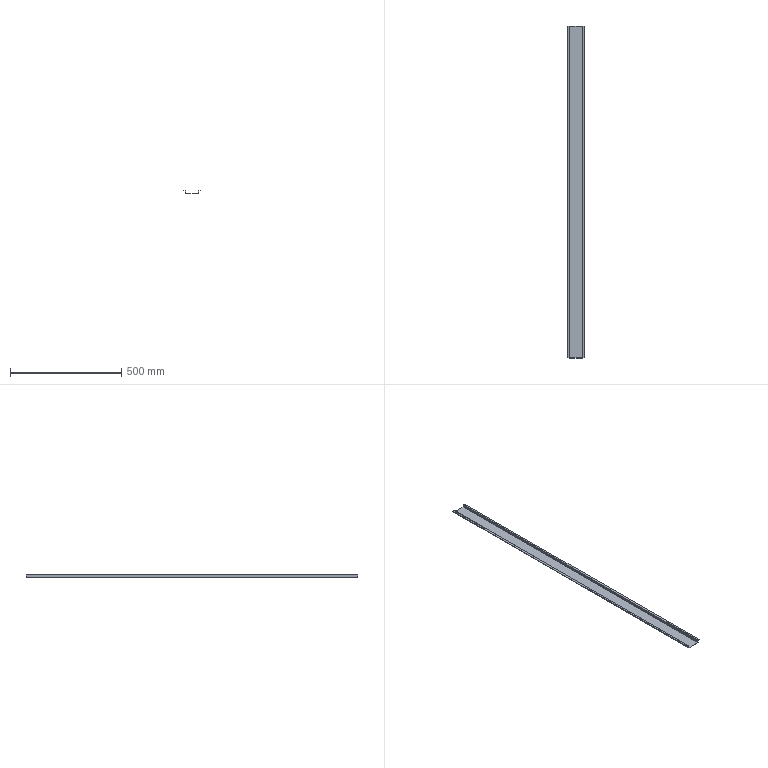Part | STEP file | HESS-408-70-15W-D-7-electrical box door panel reinforcing rib | 1 solid | 22 faces | box 77 x 1495 x 12.5 mm | volume 218735 mm3 | plane 14 | cylinder 8 | commonest cylinder face diameters 0.2 x4 3.2 x4